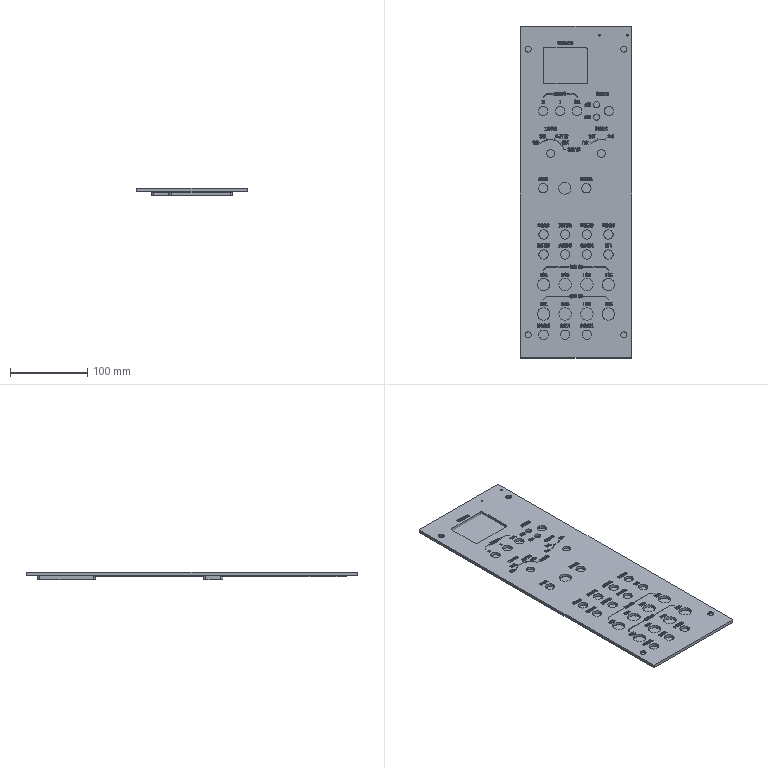NC program | Mastercam | posted with a generic post
Lines 39758 to 40600 of 54676:
(3 FEM |TOOL - 3|DIA. OFF. - 3|LEN. - 3|TOOL DIA. - 3.)
N390 T3 M6
N392 G0 G54 G90 X185. Y13. C0. B0. S10000 M3
N394 G43 H3 Z50.
N396 Z1.
N398 G1 Z0. F600.
N400 X142. Z-.623 F1000.
N402 G3 X141.5 Y12.5 Z-.635 J-.5
N404 G1 Y-40.5 Z-1.403
N406 G3 X142. Y-41. Z-1.414 I.5
N408 G1 X185. Z-2.037
N410 G3 X185.5 Y-40.5 Z-2.049 J.5
N412 G1 Y-20. Z-2.346
N414 G3 X185. Y-19.5 Z-2.357 I-.5
N416 G1 X182.5 Z-2.393
N418 G2 X177. Y-14. Z-2.518 J5.5
N420 X182.5 Y-8.5 Z-2.644 I5.5
N422 G1 X185. Z-2.68
N424 G3 X185.5 Y-8. Z-2.692 J.5
N426 G1 Y12.5 Z-2.989
N428 G3 X185. Y13. Z-3. I-.5
N430 G1 X142. Z-3.623
N432 G3 X141.5 Y12.5 Z-3.635 J-.5
N434 G1 Y-40.5 Z-4.403
N436 G3 X142. Y-41. Z-4.414 I.5
N438 G1 X185. Z-5.037
N440 G3 X185.5 Y-40.5 Z-5.049 J.5
N442 G1 Y-20. Z-5.346
N444 G3 X185. Y-19.5 Z-5.357 I-.5
N446 G1 X182.5 Z-5.393
N448 G2 X177. Y-14. Z-5.518 J5.5
N450 X182.5 Y-8.5 Z-5.644 I5.5
N452 G1 X185. Z-5.68
N454 G3 X185.5 Y-8. Z-5.692 J.5
N456 G1 Y12.5 Z-5.989
N458 G3 X185. Y13. Z-6. I-.5
N460 G1 X142. Z-6.623
N462 G3 X141.5 Y12.5 Z-6.635 J-.5
N464 G1 Y-40.5 Z-7.403
N466 G3 X142. Y-41. Z-7.414 I.5
N468 G1 X185. Z-8.037
N470 G3 X185.5 Y-40.5 Z-8.049 J.5
N472 G1 Y-20. Z-8.346
N474 G3 X185. Y-19.5 Z-8.357 I-.5
N476 G1 X182.5 Z-8.393
N478 G2 X177. Y-14. Z-8.518 J5.5
N480 X182.5 Y-8.5 Z-8.644 I5.5
N482 G1 X185. Z-8.68
N484 G3 X185.5 Y-8. Z-8.692 J.5
N486 G1 Y12.5 Z-8.989
N488 G3 X185. Y13. Z-9. I-.5
N490 G1 X142. Z-9.623
N492 G3 X141.5 Y12.5 Z-9.635 J-.5
N494 G1 Y-2.362 Z-9.85
N496 Y-40.5
N498 G3 X142. Y-41. I.5
N500 G1 X185.
N502 G3 X185.5 Y-40.5 J.5
N504 G1 Y-20.
N506 G3 X185. Y-19.5 I-.5
N508 G1 X182.5
N510 G2 X177. Y-14. J5.5
N512 X182.5 Y-8.5 I5.5
N514 G1 X185.
N516 G3 X185.5 Y-8. J.5
N518 G1 Y12.5
N520 G3 X185. Y13. I-.5
N522 G1 X142.
N524 G3 X141.5 Y12.5 J-.5
N526 G1 Y-2.362
N528 G0 Z50.
N530 X146.2 Y21.2
N532 Z1.
N534 G1 Z0. F600.
N536 X141.8 Z-.539 F1000.
N538 G3 X141.3 Y20.7 Z-.635 J-.5
N540 G1 Y18.5 Z-.904
N542 G3 X141.8 Y18. Z-1. I.5
N544 G1 X146.2 Z-1.539
N546 G3 X146.7 Y18.5 Z-1.635 J.5
N548 G1 Y20.7 Z-1.904
N550 G3 X146.2 Y21.2 Z-2. I-.5
N552 G1 X141.8 Z-2.539
N554 G3 X141.3 Y20.7 Z-2.635 J-.5
N556 G1 Y18.5 Z-2.904
N558 G3 X141.8 Y18. Z-3. I.5
N560 G1 X146.2 Z-3.539
N562 G3 X146.7 Y18.5 Z-3.635 J.5
N564 G1 Y20.7 Z-3.904
N566 G3 X146.2 Y21.2 Z-4. I-.5
N568 G1 X141.8 Z-4.539
N570 G3 X141.3 Y20.7 Z-4.635 J-.5
N572 G1 Y18.5 Z-4.904
N574 G3 X141.8 Y18. Z-5. I.5
N576 G1 X146.2 Z-5.539
N578 G3 X146.7 Y18.5 Z-5.635 J.5
N580 G1 Y20.7 Z-5.904
N582 G3 X146.2 Y21.2 Z-6. I-.5
N584 G1 X145.383 Z-6.1
N586 X141.8
N588 G3 X141.3 Y20.7 J-.5
N590 G1 Y18.5
N592 G3 X141.8 Y18. I.5
N594 G1 X146.2
N596 G3 X146.7 Y18.5 J.5
N598 G1 Y20.7
N600 G3 X146.2 Y21.2 I-.5
N602 G1 X145.383
N604 G0 Z50.
N606 X146.2 Y-46.
N608 Z1.
N610 G1 Z0. F600.
N612 X141.8 Z-.539 F1000.
N614 G3 X141.3 Y-46.5 Z-.635 J-.5
N616 G1 Y-48.7 Z-.904
N618 G3 X141.8 Y-49.2 Z-1. I.5
N620 G1 X146.2 Z-1.539
N622 G3 X146.7 Y-48.7 Z-1.635 J.5
N624 G1 Y-46.5 Z-1.904
N626 G3 X146.2 Y-46. Z-2. I-.5
N628 G1 X141.8 Z-2.539
N630 G3 X141.3 Y-46.5 Z-2.635 J-.5
N632 G1 Y-48.7 Z-2.904
N634 G3 X141.8 Y-49.2 Z-3. I.5
N636 G1 X146.2 Z-3.539
N638 G3 X146.7 Y-48.7 Z-3.635 J.5
N640 G1 Y-46.5 Z-3.904
N642 G3 X146.2 Y-46. Z-4. I-.5
N644 G1 X141.8 Z-4.539
N646 G3 X141.3 Y-46.5 Z-4.635 J-.5
N648 G1 Y-48.7 Z-4.904
N650 G3 X141.8 Y-49.2 Z-5. I.5
N652 G1 X146.2 Z-5.539
N654 G3 X146.7 Y-48.7 Z-5.635 J.5
N656 G1 Y-46.5 Z-5.904
N658 G3 X146.2 Y-46. Z-6. I-.5
N660 G1 X145.383 Z-6.1
N662 X141.8
N664 G3 X141.3 Y-46.5 J-.5
N666 G1 Y-48.7
N668 G3 X141.8 Y-49.2 I.5
N670 G1 X146.2
N672 G3 X146.7 Y-48.7 J.5
N674 G1 Y-46.5
N676 G3 X146.2 Y-46. I-.5
N678 G1 X145.383
N680 G0 Z50.
N682 X145.7 Y20.2
N684 Z-5.1
N686 G1 Z-6.1 F600.
N688 X142.3 F500.
N690 Y19.
N692 X145.7
N694 Y20.2
N696 G0 Z50.
N698 Y-47.
N700 Z-5.1
N702 G1 Z-6.1 F600.
N704 X142.3 F500.
N706 Y-48.2
N708 X145.7
N710 Y-47.
N712 G0 Z50.
N714 X50. Y29.5
N716 Z-5.
N718 G1 Z-6. F600.
N720 G3 X53.5 Y33. Z-6.063 J3.5 F3000.
N722 X50. Y36.5 Z-6.125 I-3.5
N724 X46.5 Y33. Z-6.188 J-3.5
N726 X50. Y29.5 Z-6.25 I3.5
N728 X53.5 Y33. Z-6.313 J3.5
N730 X50. Y36.5 Z-6.375 I-3.5
N732 X46.5 Y33. Z-6.438 J-3.5
N734 X50. Y29.5 Z-6.5 I3.5
N736 X53.5 Y33. Z-6.563 J3.5
N738 X50. Y36.5 Z-6.625 I-3.5
N740 X46.5 Y33. Z-6.688 J-3.5
N742 X50. Y29.5 Z-6.75 I3.5
N744 X53.5 Y33. Z-6.813 J3.5
N746 X50. Y36.5 Z-6.875 I-3.5
N748 X46.5 Y33. Z-6.938 J-3.5
N750 X50. Y29.5 Z-7. I3.5
N752 X53.5 Y33. Z-7.063 J3.5
N754 X50. Y36.5 Z-7.125 I-3.5
N756 X46.5 Y33. Z-7.188 J-3.5
N758 X50. Y29.5 Z-7.25 I3.5
N760 X53.5 Y33. Z-7.313 J3.5
N762 X50. Y36.5 Z-7.375 I-3.5
N764 X46.5 Y33. Z-7.438 J-3.5
N766 X50. Y29.5 Z-7.5 I3.5
N768 X53.5 Y33. Z-7.563 J3.5
N770 X50. Y36.5 Z-7.625 I-3.5
N772 X46.5 Y33. Z-7.688 J-3.5
N774 X50. Y29.5 Z-7.75 I3.5
N776 X53.5 Y33. Z-7.813 J3.5
N778 X50. Y36.5 Z-7.875 I-3.5
N780 X46.5 Y33. Z-7.938 J-3.5
N782 X50. Y29.5 Z-8. I3.5
N784 X53.5 Y33. Z-8.063 J3.5
N786 X50. Y36.5 Z-8.125 I-3.5
N788 X46.5 Y33. Z-8.188 J-3.5
N790 X50. Y29.5 Z-8.25 I3.5
N792 X53.5 Y33. Z-8.313 J3.5
N794 X50. Y36.5 Z-8.375 I-3.5
N796 X46.5 Y33. Z-8.438 J-3.5
N798 X50. Y29.5 Z-8.5 I3.5
N800 X53.5 Y33. Z-8.563 J3.5
N802 X50. Y36.5 Z-8.625 I-3.5
N804 X46.5 Y33. Z-8.688 J-3.5
N806 X50. Y29.5 Z-8.75 I3.5
N808 X53.5 Y33. Z-8.813 J3.5
N810 X50. Y36.5 Z-8.875 I-3.5
N812 X46.5 Y33. Z-8.938 J-3.5
N814 X50. Y29.5 Z-9. I3.5
N816 X53.5 Y33. Z-9.063 J3.5
N818 X50. Y36.5 Z-9.125 I-3.5
N820 X46.5 Y33. Z-9.188 J-3.5
N822 X50. Y29.5 Z-9.25 I3.5
N824 X53.5 Y33. Z-9.313 J3.5
N826 X50. Y36.5 Z-9.375 I-3.5
N828 X46.5 Y33. Z-9.438 J-3.5
N830 X50. Y29.5 Z-9.5 I3.5
N832 X53.5 Y33. Z-9.563 J3.5
N834 X50. Y36.5 Z-9.625 I-3.5
N836 X46.5 Y33. Z-9.688 J-3.5
N838 X50. Y29.5 Z-9.75 I3.5
N840 X53.5 Y33. Z-9.812 J3.5
N842 X52.057 Y35.832 Z-9.85 I-3.5
N844 X50. Y36.5 I-2.057 J-2.832
N846 X46.5 Y33. J-3.5
N848 X50. Y29.5 I3.5
N850 X53.5 Y33. J3.5
N852 X52.057 Y35.832 I-3.5
N854 G0 Z50.
N856 X50. Y-36.5
N858 Z-5.
N860 G1 Z-6. F600.
N862 G3 X53.5 Y-33. Z-6.063 J3.5 F3000.
N864 X50. Y-29.5 Z-6.125 I-3.5
N866 X46.5 Y-33. Z-6.188 J-3.5
N868 X50. Y-36.5 Z-6.25 I3.5
N870 X53.5 Y-33. Z-6.313 J3.5
N872 X50. Y-29.5 Z-6.375 I-3.5
N874 X46.5 Y-33. Z-6.438 J-3.5
N876 X50. Y-36.5 Z-6.5 I3.5
N878 X53.5 Y-33. Z-6.563 J3.5
N880 X50. Y-29.5 Z-6.625 I-3.5
N882 X46.5 Y-33. Z-6.688 J-3.5
N884 X50. Y-36.5 Z-6.75 I3.5
N886 X53.5 Y-33. Z-6.813 J3.5
N888 X50. Y-29.5 Z-6.875 I-3.5
N890 X46.5 Y-33. Z-6.938 J-3.5
N892 X50. Y-36.5 Z-7. I3.5
N894 X53.5 Y-33. Z-7.063 J3.5
N896 X50. Y-29.5 Z-7.125 I-3.5
N898 X46.5 Y-33. Z-7.188 J-3.5
N900 X50. Y-36.5 Z-7.25 I3.5
N902 X53.5 Y-33. Z-7.313 J3.5
N904 X50. Y-29.5 Z-7.375 I-3.5
N906 X46.5 Y-33. Z-7.438 J-3.5
N908 X50. Y-36.5 Z-7.5 I3.5
N910 X53.5 Y-33. Z-7.563 J3.5
N912 X50. Y-29.5 Z-7.625 I-3.5
N914 X46.5 Y-33. Z-7.688 J-3.5
N916 X50. Y-36.5 Z-7.75 I3.5
N918 X53.5 Y-33. Z-7.813 J3.5
N920 X50. Y-29.5 Z-7.875 I-3.5
N922 X46.5 Y-33. Z-7.938 J-3.5
N924 X50. Y-36.5 Z-8. I3.5
N926 X53.5 Y-33. Z-8.063 J3.5
N928 X50. Y-29.5 Z-8.125 I-3.5
N930 X46.5 Y-33. Z-8.188 J-3.5
N932 X50. Y-36.5 Z-8.25 I3.5
N934 X53.5 Y-33. Z-8.313 J3.5
N936 X50. Y-29.5 Z-8.375 I-3.5
N938 X46.5 Y-33. Z-8.438 J-3.5
N940 X50. Y-36.5 Z-8.5 I3.5
N942 X53.5 Y-33. Z-8.563 J3.5
N944 X50. Y-29.5 Z-8.625 I-3.5
N946 X46.5 Y-33. Z-8.688 J-3.5
N948 X50. Y-36.5 Z-8.75 I3.5
N950 X53.5 Y-33. Z-8.813 J3.5
N952 X50. Y-29.5 Z-8.875 I-3.5
N954 X46.5 Y-33. Z-8.938 J-3.5
N956 X50. Y-36.5 Z-9. I3.5
N958 X53.5 Y-33. Z-9.063 J3.5
N960 X50. Y-29.5 Z-9.125 I-3.5
N962 X46.5 Y-33. Z-9.188 J-3.5
N964 X50. Y-36.5 Z-9.25 I3.5
N966 X53.5 Y-33. Z-9.313 J3.5
N968 X50. Y-29.5 Z-9.375 I-3.5
N970 X46.5 Y-33. Z-9.438 J-3.5
N972 X50. Y-36.5 Z-9.5 I3.5
N974 X53.5 Y-33. Z-9.563 J3.5
N976 X50. Y-29.5 Z-9.625 I-3.5
N978 X46.5 Y-33. Z-9.688 J-3.5
N980 X50. Y-36.5 Z-9.75 I3.5
N982 X53.5 Y-33. Z-9.812 J3.5
N984 X52.057 Y-30.168 Z-9.85 I-3.5
N986 X50. Y-29.5 I-2.057 J-2.832
N988 X46.5 Y-33. J-3.5
N990 X50. Y-36.5 I3.5
N992 X53.5 Y-33. J3.5
N994 X52.057 Y-30.168 I-3.5
N996 G0 Z50.
N998 X109.4 Y42.5
N1000 Z-5.
N1002 G1 Z-6. F600.
N1004 G3 X105. Y46.9 Z-6.063 I-4.4 F3000.
N1006 X100.6 Y42.5 Z-6.125 J-4.4
N1008 X105. Y38.1 Z-6.188 I4.4
N1010 X109.4 Y42.5 Z-6.25 J4.4
N1012 X105. Y46.9 Z-6.313 I-4.4
N1014 X100.6 Y42.5 Z-6.375 J-4.4
N1016 X105. Y38.1 Z-6.438 I4.4
N1018 X109.4 Y42.5 Z-6.5 J4.4
N1020 X105. Y46.9 Z-6.563 I-4.4
N1022 X100.6 Y42.5 Z-6.625 J-4.4
N1024 X105. Y38.1 Z-6.688 I4.4
N1026 X109.4 Y42.5 Z-6.75 J4.4
N1028 X105. Y46.9 Z-6.813 I-4.4
N1030 X100.6 Y42.5 Z-6.875 J-4.4
N1032 X105. Y38.1 Z-6.938 I4.4
N1034 X109.4 Y42.5 Z-7. J4.4
N1036 X105. Y46.9 Z-7.063 I-4.4
N1038 X100.6 Y42.5 Z-7.125 J-4.4
N1040 X105. Y38.1 Z-7.188 I4.4
N1042 X109.4 Y42.5 Z-7.25 J4.4
N1044 X105. Y46.9 Z-7.313 I-4.4
N1046 X100.6 Y42.5 Z-7.375 J-4.4
N1048 X105. Y38.1 Z-7.438 I4.4
N1050 X109.4 Y42.5 Z-7.5 J4.4
N1052 X105. Y46.9 Z-7.563 I-4.4
N1054 X100.6 Y42.5 Z-7.625 J-4.4
N1056 X105. Y38.1 Z-7.688 I4.4
N1058 X109.4 Y42.5 Z-7.75 J4.4
N1060 X105. Y46.9 Z-7.813 I-4.4
N1062 X100.6 Y42.5 Z-7.875 J-4.4
N1064 X105. Y38.1 Z-7.938 I4.4
N1066 X109.4 Y42.5 Z-8. J4.4
N1068 X105. Y46.9 Z-8.063 I-4.4
N1070 X100.6 Y42.5 Z-8.125 J-4.4
N1072 X105. Y38.1 Z-8.188 I4.4
N1074 X109.4 Y42.5 Z-8.25 J4.4
N1076 X105. Y46.9 Z-8.313 I-4.4
N1078 X100.6 Y42.5 Z-8.375 J-4.4
N1080 X105. Y38.1 Z-8.438 I4.4
N1082 X109.4 Y42.5 Z-8.5 J4.4
N1084 X105. Y46.9 Z-8.563 I-4.4
N1086 X100.6 Y42.5 Z-8.625 J-4.4
N1088 X105. Y38.1 Z-8.688 I4.4
N1090 X109.4 Y42.5 Z-8.75 J4.4
N1092 X105. Y46.9 Z-8.813 I-4.4
N1094 X100.6 Y42.5 Z-8.875 J-4.4
N1096 X105. Y38.1 Z-8.938 I4.4
N1098 X109.4 Y42.5 Z-9. J4.4
N1100 X105. Y46.9 Z-9.063 I-4.4
N1102 X100.6 Y42.5 Z-9.125 J-4.4
N1104 X105. Y38.1 Z-9.188 I4.4
N1106 X109.4 Y42.5 Z-9.25 J4.4
N1108 X105. Y46.9 Z-9.313 I-4.4
N1110 X100.6 Y42.5 Z-9.375 J-4.4
N1112 X105. Y38.1 Z-9.438 I4.4
N1114 X109.4 Y42.5 Z-9.5 J4.4
N1116 X105. Y46.9 Z-9.563 I-4.4
N1118 X100.6 Y42.5 Z-9.625 J-4.4
N1120 X105. Y38.1 Z-9.688 I4.4
N1122 X109.4 Y42.5 Z-9.75 J4.4
N1124 X105. Y46.9 Z-9.812 I-4.4
N1126 X101.44 Y45.086 Z-9.85 J-4.4
N1128 X100.6 Y42.5 I3.56 J-2.586
N1130 X105. Y38.1 I4.4
N1132 X109.4 Y42.5 J4.4
N1134 X105. Y46.9 I-4.4
N1136 X101.44 Y45.086 J-4.4
N1138 G0 Z50.
N1140 X5. Y18.
N1142 Z-5.
N1144 G1 Z-6. F600.
N1146 G3 X.5 Y13.5 Z-6.063 J-4.5 F3000.
N1148 X5. Y9. Z-6.125 I4.5
N1150 X9.5 Y13.5 Z-6.188 J4.5
N1152 X5. Y18. Z-6.25 I-4.5
N1154 X.5 Y13.5 Z-6.313 J-4.5
N1156 X5. Y9. Z-6.375 I4.5
N1158 X9.5 Y13.5 Z-6.438 J4.5
N1160 X5. Y18. Z-6.5 I-4.5
N1162 X.5 Y13.5 Z-6.563 J-4.5
N1164 X5. Y9. Z-6.625 I4.5
N1166 X9.5 Y13.5 Z-6.688 J4.5
N1168 X5. Y18. Z-6.75 I-4.5
N1170 X.5 Y13.5 Z-6.813 J-4.5
N1172 X5. Y9. Z-6.875 I4.5
N1174 X9.5 Y13.5 Z-6.938 J4.5
N1176 X5. Y18. Z-7. I-4.5
N1178 X.5 Y13.5 Z-7.063 J-4.5
N1180 X5. Y9. Z-7.125 I4.5
N1182 X9.5 Y13.5 Z-7.188 J4.5
N1184 X5. Y18. Z-7.25 I-4.5
N1186 X.5 Y13.5 Z-7.313 J-4.5
N1188 X5. Y9. Z-7.375 I4.5
N1190 X9.5 Y13.5 Z-7.438 J4.5
N1192 X5. Y18. Z-7.5 I-4.5
N1194 X.5 Y13.5 Z-7.563 J-4.5
N1196 X5. Y9. Z-7.625 I4.5
N1198 X9.5 Y13.5 Z-7.688 J4.5
N1200 X5. Y18. Z-7.75 I-4.5
N1202 X.5 Y13.5 Z-7.813 J-4.5
N1204 X5. Y9. Z-7.875 I4.5
N1206 X9.5 Y13.5 Z-7.938 J4.5
N1208 X5. Y18. Z-8. I-4.5
N1210 X.5 Y13.5 Z-8.063 J-4.5
N1212 X5. Y9. Z-8.125 I4.5
N1214 X9.5 Y13.5 Z-8.188 J4.5
N1216 X5. Y18. Z-8.25 I-4.5
N1218 X.5 Y13.5 Z-8.313 J-4.5
N1220 X5. Y9. Z-8.375 I4.5
N1222 X9.5 Y13.5 Z-8.438 J4.5
N1224 X5. Y18. Z-8.5 I-4.5
N1226 X.5 Y13.5 Z-8.563 J-4.5
N1228 X5. Y9. Z-8.625 I4.5
N1230 X9.5 Y13.5 Z-8.688 J4.5
N1232 X5. Y18. Z-8.75 I-4.5
N1234 X.5 Y13.5 Z-8.813 J-4.5
N1236 X5. Y9. Z-8.875 I4.5
N1238 X9.5 Y13.5 Z-8.938 J4.5
N1240 X5. Y18. Z-9. I-4.5
N1242 X.5 Y13.5 Z-9.063 J-4.5
N1244 X5. Y9. Z-9.125 I4.5
N1246 X9.5 Y13.5 Z-9.188 J4.5
N1248 X5. Y18. Z-9.25 I-4.5
N1250 X.5 Y13.5 Z-9.313 J-4.5
N1252 X5. Y9. Z-9.375 I4.5
N1254 X9.5 Y13.5 Z-9.438 J4.5
N1256 X5. Y18. Z-9.5 I-4.5
N1258 X.5 Y13.5 Z-9.563 J-4.5
N1260 X5. Y9. Z-9.625 I4.5
N1262 X9.5 Y13.5 Z-9.688 J4.5
N1264 X5. Y18. Z-9.75 I-4.5
N1266 X.5 Y13.5 Z-9.813 J-4.5
N1268 X2.355 Y9.859 Z-9.85 I4.5
N1270 X5. Y9. I2.645 J3.641
N1272 X9.5 Y13.5 J4.5
N1274 X5. Y18. I-4.5
N1276 X.5 Y13.5 J-4.5
N1278 X2.355 Y9.859 I4.5
N1280 G0 Z50.
N1282 X5. Y-8.1
N1284 Z-5.
N1286 G1 Z-6. F600.
N1288 G3 X-1.4 Y-14.5 Z-6.063 J-6.4 F3000.
N1290 X5. Y-20.9 Z-6.125 I6.4
N1292 X11.4 Y-14.5 Z-6.188 J6.4
N1294 X5. Y-8.1 Z-6.25 I-6.4
N1296 X-1.4 Y-14.5 Z-6.313 J-6.4
N1298 X5. Y-20.9 Z-6.375 I6.4
N1300 X11.4 Y-14.5 Z-6.438 J6.4
N1302 X5. Y-8.1 Z-6.5 I-6.4
N1304 X-1.4 Y-14.5 Z-6.563 J-6.4
N1306 X5. Y-20.9 Z-6.625 I6.4
N1308 X11.4 Y-14.5 Z-6.688 J6.4
N1310 X5. Y-8.1 Z-6.75 I-6.4
N1312 X-1.4 Y-14.5 Z-6.813 J-6.4
N1314 X5. Y-20.9 Z-6.875 I6.4
N1316 X11.4 Y-14.5 Z-6.938 J6.4
N1318 X5. Y-8.1 Z-7. I-6.4
N1320 X-1.4 Y-14.5 Z-7.063 J-6.4
N1322 X5. Y-20.9 Z-7.125 I6.4
N1324 X11.4 Y-14.5 Z-7.188 J6.4
N1326 X5. Y-8.1 Z-7.25 I-6.4
N1328 X-1.4 Y-14.5 Z-7.313 J-6.4
N1330 X5. Y-20.9 Z-7.375 I6.4
N1332 X11.4 Y-14.5 Z-7.438 J6.4
N1334 X5. Y-8.1 Z-7.5 I-6.4
N1336 X-1.4 Y-14.5 Z-7.563 J-6.4
N1338 X5. Y-20.9 Z-7.625 I6.4
N1340 X11.4 Y-14.5 Z-7.688 J6.4
N1342 X5. Y-8.1 Z-7.75 I-6.4
N1344 X-1.4 Y-14.5 Z-7.813 J-6.4
N1346 X5. Y-20.9 Z-7.875 I6.4
N1348 X11.4 Y-14.5 Z-7.938 J6.4
N1350 X5. Y-8.1 Z-8. I-6.4
N1352 X-1.4 Y-14.5 Z-8.063 J-6.4
N1354 X5. Y-20.9 Z-8.125 I6.4
N1356 X11.4 Y-14.5 Z-8.188 J6.4
N1358 X5. Y-8.1 Z-8.25 I-6.4
N1360 X-1.4 Y-14.5 Z-8.313 J-6.4
N1362 X5. Y-20.9 Z-8.375 I6.4
N1364 X11.4 Y-14.5 Z-8.438 J6.4
N1366 X5. Y-8.1 Z-8.5 I-6.4
N1368 X-1.4 Y-14.5 Z-8.563 J-6.4
N1370 X5. Y-20.9 Z-8.625 I6.4
N1372 X11.4 Y-14.5 Z-8.688 J6.4
N1374 X5. Y-8.1 Z-8.75 I-6.4
N1376 X-1.4 Y-14.5 Z-8.813 J-6.4
N1378 X5. Y-20.9 Z-8.875 I6.4
N1380 X11.4 Y-14.5 Z-8.938 J6.4
N1382 X5. Y-8.1 Z-9. I-6.4
N1384 X-1.4 Y-14.5 Z-9.063 J-6.4
N1386 X5. Y-20.9 Z-9.125 I6.4
N1388 X11.4 Y-14.5 Z-9.188 J6.4
N1390 X5. Y-8.1 Z-9.25 I-6.4
N1392 X-1.4 Y-14.5 Z-9.313 J-6.4
N1394 X5. Y-20.9 Z-9.375 I6.4
N1396 X11.4 Y-14.5 Z-9.438 J6.4
N1398 X5. Y-8.1 Z-9.5 I-6.4
N1400 X-1.4 Y-14.5 Z-9.563 J-6.4
N1402 X5. Y-20.9 Z-9.625 I6.4
N1404 X11.4 Y-14.5 Z-9.688 J6.4
N1406 X5. Y-8.1 Z-9.75 I-6.4
N1408 X-1.4 Y-14.5 Z-9.812 J-6.4
N1410 X1.238 Y-19.678 Z-9.85 I6.4
N1412 X5. Y-20.9 I3.762 J5.178
N1414 X11.4 Y-14.5 J6.4
N1416 X5. Y-8.1 I-6.4
N1418 X-1.4 Y-14.5 J-6.4
N1420 X1.238 Y-19.678 I6.4
N1422 G0 Z50.
N1424 X5. Y-38.
N1426 Z-5.
N1428 G1 Z-6. F600.
N1430 G3 X.5 Y-42.5 Z-6.063 J-4.5 F3000.
N1432 X5. Y-47. Z-6.125 I4.5
N1434 X9.5 Y-42.5 Z-6.188 J4.5
N1436 X5. Y-38. Z-6.25 I-4.5
N1438 X.5 Y-42.5 Z-6.313 J-4.5
N1440 X5. Y-47. Z-6.375 I4.5
N1442 X9.5 Y-42.5 Z-6.438 J4.5
N1444 X5. Y-38. Z-6.5 I-4.5
N1446 X.5 Y-42.5 Z-6.563 J-4.5
N1448 X5. Y-47. Z-6.625 I4.5
N1450 X9.5 Y-42.5 Z-6.688 J4.5
N1452 X5. Y-38. Z-6.75 I-4.5
N1454 X.5 Y-42.5 Z-6.813 J-4.5
N1456 X5. Y-47. Z-6.875 I4.5
N1458 X9.5 Y-42.5 Z-6.938 J4.5
N1460 X5. Y-38. Z-7. I-4.5
N1462 X.5 Y-42.5 Z-7.063 J-4.5
N1464 X5. Y-47. Z-7.125 I4.5
N1466 X9.5 Y-42.5 Z-7.188 J4.5
N1468 X5. Y-38. Z-7.25 I-4.5
N1470 X.5 Y-42.5 Z-7.313 J-4.5
N1472 X5. Y-47. Z-7.375 I4.5
N1474 X9.5 Y-42.5 Z-7.438 J4.5
N1476 X5. Y-38. Z-7.5 I-4.5
N1478 X.5 Y-42.5 Z-7.563 J-4.5
N1480 X5. Y-47. Z-7.625 I4.5
N1482 X9.5 Y-42.5 Z-7.688 J4.5
N1484 X5. Y-38. Z-7.75 I-4.5
N1486 X.5 Y-42.5 Z-7.813 J-4.5
N1488 X5. Y-47. Z-7.875 I4.5
N1490 X9.5 Y-42.5 Z-7.938 J4.5
N1492 X5. Y-38. Z-8. I-4.5
N1494 X.5 Y-42.5 Z-8.063 J-4.5
N1496 X5. Y-47. Z-8.125 I4.5
N1498 X9.5 Y-42.5 Z-8.188 J4.5
N1500 X5. Y-38. Z-8.25 I-4.5
N1502 X.5 Y-42.5 Z-8.313 J-4.5
N1504 X5. Y-47. Z-8.375 I4.5
N1506 X9.5 Y-42.5 Z-8.438 J4.5
N1508 X5. Y-38. Z-8.5 I-4.5
N1510 X.5 Y-42.5 Z-8.563 J-4.5
N1512 X5. Y-47. Z-8.625 I4.5
N1514 X9.5 Y-42.5 Z-8.688 J4.5
N1516 X5. Y-38. Z-8.75 I-4.5
N1518 X.5 Y-42.5 Z-8.813 J-4.5
N1520 X5. Y-47. Z-8.875 I4.5
N1522 X9.5 Y-42.5 Z-8.938 J4.5
N1524 X5. Y-38. Z-9. I-4.5
N1526 X.5 Y-42.5 Z-9.063 J-4.5
N1528 X5. Y-47. Z-9.125 I4.5
N1530 X9.5 Y-42.5 Z-9.188 J4.5
N1532 X5. Y-38. Z-9.25 I-4.5
N1534 X.5 Y-42.5 Z-9.313 J-4.5
N1536 X5. Y-47. Z-9.375 I4.5
N1538 X9.5 Y-42.5 Z-9.438 J4.5
N1540 X5. Y-38. Z-9.5 I-4.5
N1542 X.5 Y-42.5 Z-9.563 J-4.5
N1544 X5. Y-47. Z-9.625 I4.5
N1546 X9.5 Y-42.5 Z-9.688 J4.5
N1548 X5. Y-38. Z-9.75 I-4.5
N1550 X.5 Y-42.5 Z-9.813 J-4.5
N1552 X2.355 Y-46.141 Z-9.85 I4.5
N1554 X5. Y-47. I2.645 J3.641
N1556 X9.5 Y-42.5 J4.5
N1558 X5. Y-38. I-4.5
N1560 X.5 Y-42.5 J-4.5
N1562 X2.355 Y-46.141 I4.5
N1564 G0 Z50.
N1566 X105. Y6.
N1568 Z-5.
N1570 G1 Z-6. F600.
N1572 G3 X100.5 Y1.5 Z-6.063 J-4.5 F3000.
N1574 X105. Y-3. Z-6.125 I4.5
N1576 X109.5 Y1.5 Z-6.188 J4.5
N1578 X105. Y6. Z-6.25 I-4.5
N1580 X100.5 Y1.5 Z-6.313 J-4.5
N1582 X105. Y-3. Z-6.375 I4.5
N1584 X109.5 Y1.5 Z-6.438 J4.5
N1586 X105. Y6. Z-6.5 I-4.5
N1588 X100.5 Y1.5 Z-6.563 J-4.5
N1590 X105. Y-3. Z-6.625 I4.5
N1592 X109.5 Y1.5 Z-6.688 J4.5
N1594 X105. Y6. Z-6.75 I-4.5
N1596 X100.5 Y1.5 Z-6.813 J-4.5
N1598 X105. Y-3. Z-6.875 I4.5
N1600 X109.5 Y1.5 Z-6.938 J4.5
N1602 X105. Y6. Z-7. I-4.5
N1604 X100.5 Y1.5 Z-7.063 J-4.5
N1606 X105. Y-3. Z-7.125 I4.5
N1608 X109.5 Y1.5 Z-7.188 J4.5
N1610 X105. Y6. Z-7.25 I-4.5
N1612 X100.5 Y1.5 Z-7.313 J-4.5
N1614 X105. Y-3. Z-7.375 I4.5
N1616 X109.5 Y1.5 Z-7.438 J4.5
N1618 X105. Y6. Z-7.5 I-4.5
N1620 X100.5 Y1.5 Z-7.563 J-4.5
N1622 X105. Y-3. Z-7.625 I4.5
N1624 X109.5 Y1.5 Z-7.688 J4.5
N1626 X105. Y6. Z-7.75 I-4.5
N1628 X100.5 Y1.5 Z-7.813 J-4.5
N1630 X105. Y-3. Z-7.875 I4.5
N1632 X109.5 Y1.5 Z-7.938 J4.5
N1634 X105. Y6. Z-8. I-4.5
N1636 X100.5 Y1.5 Z-8.063 J-4.5
N1638 X105. Y-3. Z-8.125 I4.5
N1640 X109.5 Y1.5 Z-8.188 J4.5
N1642 X105. Y6. Z-8.25 I-4.5
N1644 X100.5 Y1.5 Z-8.313 J-4.5
N1646 X105. Y-3. Z-8.375 I4.5
N1648 X109.5 Y1.5 Z-8.438 J4.5
N1650 X105. Y6. Z-8.5 I-4.5
N1652 X100.5 Y1.5 Z-8.563 J-4.5
N1654 X105. Y-3. Z-8.625 I4.5
N1656 X109.5 Y1.5 Z-8.688 J4.5
N1658 X105. Y6. Z-8.75 I-4.5
N1660 X100.5 Y1.5 Z-8.813 J-4.5
N1662 X105. Y-3. Z-8.875 I4.5
N1664 X109.5 Y1.5 Z-8.938 J4.5
N1666 X105. Y6. Z-9. I-4.5
N1668 X100.5 Y1.5 Z-9.063 J-4.5
N1670 X105. Y-3. Z-9.125 I4.5
N1672 X109.5 Y1.5 Z-9.188 J4.5
N1674 X105. Y6. Z-9.25 I-4.5
N1676 X100.5 Y1.5 Z-9.313 J-4.5
N1678 X105. Y-3. Z-9.375 I4.5
N1680 X109.5 Y1.5 Z-9.438 J4.5
N1682 X105. Y6. Z-9.5 I-4.5
N1684 X100.5 Y1.5 Z-9.563 J-4.5
N1686 X105. Y-3. Z-9.625 I4.5
N1688 X109.5 Y1.5 Z-9.688 J4.5
N1690 X105. Y6. Z-9.75 I-4.5
N1692 X100.5 Y1.5 Z-9.813 J-4.5
N1694 X102.355 Y-2.141 Z-9.85 I4.5
N1696 X105. Y-3. I2.645 J3.641
N1698 X109.5 Y1.5 J4.5
N1700 X105. Y6. I-4.5
N1702 X100.5 Y1.5 J-4.5
N1704 X102.355 Y-2.141 I4.5
N1706 G0 Z50.
N1708 X105. Y-16.
N1710 Z-5.
N1712 G1 Z-6. F600.
N1714 G3 X100.5 Y-20.5 Z-6.063 J-4.5 F3000.
N1716 X105. Y-25. Z-6.125 I4.5
N1718 X109.5 Y-20.5 Z-6.188 J4.5
N1720 X105. Y-16. Z-6.25 I-4.5
N1722 X100.5 Y-20.5 Z-6.313 J-4.5
N1724 X105. Y-25. Z-6.375 I4.5
N1726 X109.5 Y-20.5 Z-6.438 J4.5
N1728 X105. Y-16. Z-6.5 I-4.5
N1730 X100.5 Y-20.5 Z-6.563 J-4.5
N1732 X105. Y-25. Z-6.625 I4.5
N1734 X109.5 Y-20.5 Z-6.688 J4.5
N1736 X105. Y-16. Z-6.75 I-4.5
N1738 X100.5 Y-20.5 Z-6.813 J-4.5
N1740 X105. Y-25. Z-6.875 I4.5
N1742 X109.5 Y-20.5 Z-6.938 J4.5
N1744 X105. Y-16. Z-7. I-4.5
N1746 X100.5 Y-20.5 Z-7.063 J-4.5
N1748 X105. Y-25. Z-7.125 I4.5
N1750 X109.5 Y-20.5 Z-7.188 J4.5
N1752 X105. Y-16. Z-7.25 I-4.5
N1754 X100.5 Y-20.5 Z-7.313 J-4.5
N1756 X105. Y-25. Z-7.375 I4.5
N1758 X109.5 Y-20.5 Z-7.438 J4.5
N1760 X105. Y-16. Z-7.5 I-4.5
N1762 X100.5 Y-20.5 Z-7.563 J-4.5
N1764 X105. Y-25. Z-7.625 I4.5
N1766 X109.5 Y-20.5 Z-7.688 J4.5
N1768 X105. Y-16. Z-7.75 I-4.5
N1770 X100.5 Y-20.5 Z-7.813 J-4.5
N1772 X105. Y-25. Z-7.875 I4.5
N1774 X109.5 Y-20.5 Z-7.938 J4.5
N1776 X105. Y-16. Z-8. I-4.5
N1778 X100.5 Y-20.5 Z-8.063 J-4.5
N1780 X105. Y-25. Z-8.125 I4.5
N1782 X109.5 Y-20.5 Z-8.188 J4.5
N1784 X105. Y-16. Z-8.25 I-4.5
N1786 X100.5 Y-20.5 Z-8.313 J-4.5
N1788 X105. Y-25. Z-8.375 I4.5
N1790 X109.5 Y-20.5 Z-8.438 J4.5
N1792 X105. Y-16. Z-8.5 I-4.5
N1794 X100.5 Y-20.5 Z-8.563 J-4.5
N1796 X105. Y-25. Z-8.625 I4.5
N1798 X109.5 Y-20.5 Z-8.688 J4.5
N1800 X105. Y-16. Z-8.75 I-4.5
N1802 X100.5 Y-20.5 Z-8.813 J-4.5
N1804 X105. Y-25. Z-8.875 I4.5
N1806 X109.5 Y-20.5 Z-8.938 J4.5
N1808 X105. Y-16. Z-9. I-4.5
N1810 X100.5 Y-20.5 Z-9.063 J-4.5
N1812 X105. Y-25. Z-9.125 I4.5
N1814 X109.5 Y-20.5 Z-9.188 J4.5
N1816 X105. Y-16. Z-9.25 I-4.5
N1818 X100.5 Y-20.5 Z-9.313 J-4.5
N1820 X105. Y-25. Z-9.375 I4.5
N1822 X109.5 Y-20.5 Z-9.438 J4.5
N1824 X105. Y-16. Z-9.5 I-4.5
N1826 X100.5 Y-20.5 Z-9.563 J-4.5
N1828 X105. Y-25. Z-9.625 I4.5
N1830 X109.5 Y-20.5 Z-9.688 J4.5
N1832 X105. Y-16. Z-9.75 I-4.5
N1834 X100.5 Y-20.5 Z-9.813 J-4.5
N1836 X102.355 Y-24.141 Z-9.85 I4.5
N1838 X105. Y-25. I2.645 J3.641
N1840 X109.5 Y-20.5 J4.5
N1842 X105. Y-16. I-4.5
N1844 X100.5 Y-20.5 J-4.5
N1846 X102.355 Y-24.141 I4.5
N1848 G0 Z50.
N1850 X105. Y-38.
N1852 Z-5.
N1854 G1 Z-6. F600.
N1856 G3 X100.5 Y-42.5 Z-6.063 J-4.5 F3000.
N1858 X105. Y-47. Z-6.125 I4.5
N1860 X109.5 Y-42.5 Z-6.188 J4.5
N1862 X105. Y-38. Z-6.25 I-4.5
N1864 X100.5 Y-42.5 Z-6.313 J-4.5
N1866 X105. Y-47. Z-6.375 I4.5
N1868 X109.5 Y-42.5 Z-6.438 J4.5
N1870 X105. Y-38. Z-6.5 I-4.5
N1872 X100.5 Y-42.5 Z-6.563 J-4.5
N1874 X105. Y-47. Z-6.625 I4.5
N1876 X109.5 Y-42.5 Z-6.688 J4.5
N1878 X105. Y-38. Z-6.75 I-4.5
N1880 X100.5 Y-42.5 Z-6.813 J-4.5
N1882 X105. Y-47. Z-6.875 I4.5
N1884 X109.5 Y-42.5 Z-6.938 J4.5
N1886 X105. Y-38. Z-7. I-4.5
N1888 X100.5 Y-42.5 Z-7.063 J-4.5
N1890 X105. Y-47. Z-7.125 I4.5
N1892 X109.5 Y-42.5 Z-7.188 J4.5
N1894 X105. Y-38. Z-7.25 I-4.5
N1896 X100.5 Y-42.5 Z-7.313 J-4.5
N1898 X105. Y-47. Z-7.375 I4.5
N1900 X109.5 Y-42.5 Z-7.438 J4.5
N1902 X105. Y-38. Z-7.5 I-4.5
N1904 X100.5 Y-42.5 Z-7.563 J-4.5
N1906 X105. Y-47. Z-7.625 I4.5
N1908 X109.5 Y-42.5 Z-7.688 J4.5
N1910 X105. Y-38. Z-7.75 I-4.5
N1912 X100.5 Y-42.5 Z-7.813 J-4.5
N1914 X105. Y-47. Z-7.875 I4.5
N1916 X109.5 Y-42.5 Z-7.938 J4.5
N1918 X105. Y-38. Z-8. I-4.5
N1920 X100.5 Y-42.5 Z-8.063 J-4.5
N1922 X105. Y-47. Z-8.125 I4.5
N1924 X109.5 Y-42.5 Z-8.188 J4.5
N1926 X105. Y-38. Z-8.25 I-4.5
N1928 X100.5 Y-42.5 Z-8.313 J-4.5
N1930 X105. Y-47. Z-8.375 I4.5
N1932 X109.5 Y-42.5 Z-8.438 J4.5
N1934 X105. Y-38. Z-8.5 I-4.5
N1936 X100.5 Y-42.5 Z-8.563 J-4.5
N1938 X105. Y-47. Z-8.625 I4.5
N1940 X109.5 Y-42.5 Z-8.688 J4.5
N1942 X105. Y-38. Z-8.75 I-4.5
N1944 X100.5 Y-42.5 Z-8.813 J-4.5
N1946 X105. Y-47. Z-8.875 I4.5
N1948 X109.5 Y-42.5 Z-8.938 J4.5
N1950 X105. Y-38. Z-9. I-4.5
N1952 X100.5 Y-42.5 Z-9.063 J-4.5
N1954 X105. Y-47. Z-9.125 I4.5
N1956 X109.5 Y-42.5 Z-9.188 J4.5
N1958 X105. Y-38. Z-9.25 I-4.5
N1960 X100.5 Y-42.5 Z-9.313 J-4.5
N1962 X105. Y-47. Z-9.375 I4.5
N1964 X109.5 Y-42.5 Z-9.438 J4.5
N1966 X105. Y-38. Z-9.5 I-4.5
N1968 X100.5 Y-42.5 Z-9.563 J-4.5
N1970 X105. Y-47. Z-9.625 I4.5
N1972 X109.5 Y-42.5 Z-9.688 J4.5
N1974 X105. Y-38. Z-9.75 I-4.5
N1976 X100.5 Y-42.5 Z-9.813 J-4.5
N1978 X102.355 Y-46.141 Z-9.85 I4.5
N1980 X105. Y-47. I2.645 J3.641
N1982 X109.5 Y-42.5 J4.5
N1984 X105. Y-38. I-4.5
N1986 X100.5 Y-42.5 J-4.5
N1988 X102.355 Y-46.141 I4.5
N1990 G0 Z50.
N1992 X-55. Y-37.5
N1994 Z-5.
N1996 G1 Z-6. F600.
N1998 G3 X-59.5 Y-42. Z-6.063 J-4.5 F3000.
N2000 X-55. Y-46.5 Z-6.125 I4.5
N2002 X-50.5 Y-42. Z-6.188 J4.5
N2004 X-55. Y-37.5 Z-6.25 I-4.5
N2006 X-59.5 Y-42. Z-6.313 J-4.5
N2008 X-55. Y-46.5 Z-6.375 I4.5
N2010 X-50.5 Y-42. Z-6.438 J4.5
N2012 X-55. Y-37.5 Z-6.5 I-4.5
N2014 X-59.5 Y-42. Z-6.563 J-4.5
N2016 X-55. Y-46.5 Z-6.625 I4.5
N2018 X-50.5 Y-42. Z-6.688 J4.5
N2020 X-55. Y-37.5 Z-6.75 I-4.5
N2022 X-59.5 Y-42. Z-6.813 J-4.5
N2024 X-55. Y-46.5 Z-6.875 I4.5
N2026 X-50.5 Y-42. Z-6.938 J4.5
N2028 X-55. Y-37.5 Z-7. I-4.5
N2030 X-59.5 Y-42. Z-7.063 J-4.5
N2032 X-55. Y-46.5 Z-7.125 I4.5
N2034 X-50.5 Y-42. Z-7.188 J4.5
N2036 X-55. Y-37.5 Z-7.25 I-4.5
N2038 X-59.5 Y-42. Z-7.313 J-4.5
N2040 X-55. Y-46.5 Z-7.375 I4.5
N2042 X-50.5 Y-42. Z-7.438 J4.5
N2044 X-55. Y-37.5 Z-7.5 I-4.5
N2046 X-59.5 Y-42. Z-7.563 J-4.5
N2048 X-55. Y-46.5 Z-7.625 I4.5
N2050 X-50.5 Y-42. Z-7.688 J4.5
N2052 X-55. Y-37.5 Z-7.75 I-4.5
N2054 X-59.5 Y-42. Z-7.813 J-4.5
N2056 X-55. Y-46.5 Z-7.875 I4.5
N2058 X-50.5 Y-42. Z-7.938 J4.5
N2060 X-55. Y-37.5 Z-8. I-4.5
N2062 X-59.5 Y-42. Z-8.063 J-4.5
N2064 X-55. Y-46.5 Z-8.125 I4.5
N2066 X-50.5 Y-42. Z-8.188 J4.5
N2068 X-55. Y-37.5 Z-8.25 I-4.5
N2070 X-59.5 Y-42. Z-8.313 J-4.5
N2072 X-55. Y-46.5 Z-8.375 I4.5